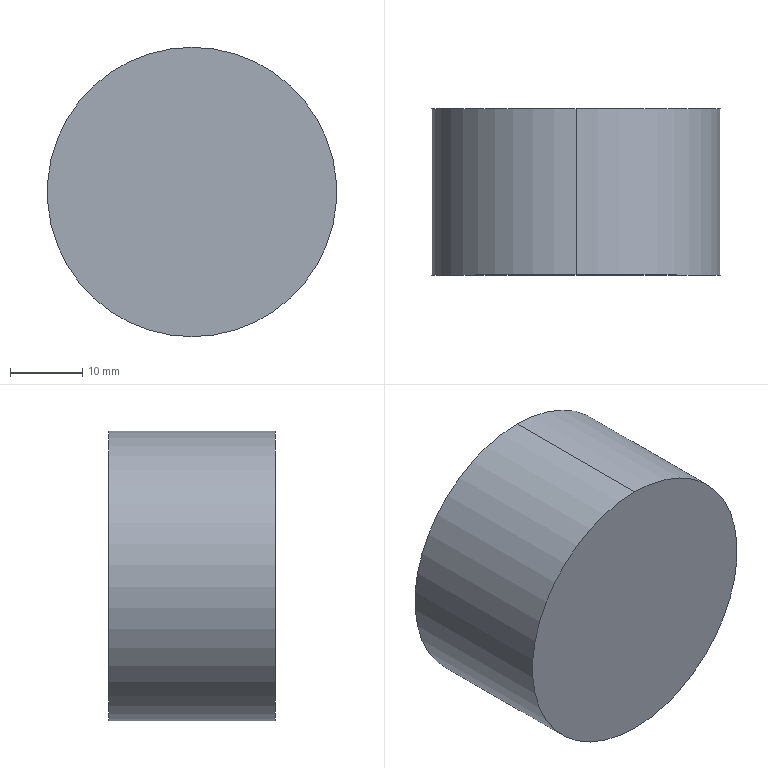Part | 1 solid | 4 faces | box 40 x 23 x 40 mm | volume 28903 mm3 | cylinder 2 | plane 2 | commonest cylinder face diameters 40 x2
STEP:
#1=CARTESIAN_POINT('',(0.,0.,0.));
#2=DIRECTION('',(0.,0.,1.));
#3=DIRECTION('',(1.,0.,0.));
#4=AXIS2_PLACEMENT_3D('',#1,#2,#3);
#5=CARTESIAN_POINT('',(-239.028,-123.5,-320.55));
#6=VERTEX_POINT('',#5);
#7=CARTESIAN_POINT('',(-239.028,-100.5,-320.55));
#8=VERTEX_POINT('',#7);
#9=CARTESIAN_POINT('',(-239.028,-123.5,-320.55));
#10=DIRECTION('',(0.,1.,0.));
#11=VECTOR('',#10,1.);
#12=LINE('',#9,#11);
#13=CARTESIAN_POINT('',(-239.028,-123.5,-300.55));
#14=DIRECTION('',(0.,1.,0.));
#15=DIRECTION('',(1.,0.,0.));
#16=AXIS2_PLACEMENT_3D('',#13,#14,#15);
#17=CYLINDRICAL_SURFACE('',#16,20.);
#18=CARTESIAN_POINT('',(1.571,0.));
#19=DIRECTION('',(0.,1.));
#20=VECTOR('',#19,1.);
#21=LINE('',#18,#20);
#22=(GEOMETRIC_REPRESENTATION_CONTEXT(2)PARAMETRIC_REPRESENTATION_CONTEXT()REPRESENTATION_CONTEXT('',''));
#23=DEFINITIONAL_REPRESENTATION('',(#21),#22);
#24=PCURVE('',#17,#23);
#25=CARTESIAN_POINT('',(-239.028,-123.5,-300.55));
#26=DIRECTION('',(0.,1.,0.));
#27=DIRECTION('',(-1.,0.,0.));
#28=AXIS2_PLACEMENT_3D('',#25,#26,#27);
#29=CYLINDRICAL_SURFACE('',#28,20.);
#30=CARTESIAN_POINT('',(4.712,0.));
#31=DIRECTION('',(0.,1.));
#32=VECTOR('',#31,1.);
#33=LINE('',#30,#32);
#34=(GEOMETRIC_REPRESENTATION_CONTEXT(2)PARAMETRIC_REPRESENTATION_CONTEXT()REPRESENTATION_CONTEXT('',''));
#35=DEFINITIONAL_REPRESENTATION('',(#33),#34);
#36=PCURVE('',#29,#35);
#37=SURFACE_CURVE('',#12,(#24,#36),.PCURVE_S1.);
#38=EDGE_CURVE('',#6,#8,#37,.T.);
#39=ORIENTED_EDGE('',*,*,#38,.F.);
#40=CARTESIAN_POINT('',(-239.028,-123.5,-280.55));
#41=VERTEX_POINT('',#40);
#42=CARTESIAN_POINT('',(-239.028,-123.5,-300.55));
#43=DIRECTION('',(0.,-1.,0.));
#44=DIRECTION('',(0.,0.,1.));
#45=AXIS2_PLACEMENT_3D('',#42,#43,#44);
#46=CIRCLE('',#45,20.);
#47=CARTESIAN_POINT('',(4.712,0.));
#48=DIRECTION('',(-1.,0.));
#49=VECTOR('',#48,1.);
#50=LINE('',#47,#49);
#51=(GEOMETRIC_REPRESENTATION_CONTEXT(2)PARAMETRIC_REPRESENTATION_CONTEXT()REPRESENTATION_CONTEXT('',''));
#52=DEFINITIONAL_REPRESENTATION('',(#50),#51);
#53=PCURVE('',#17,#52);
#54=CARTESIAN_POINT('',(-239.028,-123.5,-300.55));
#55=DIRECTION('',(0.,-1.,0.));
#56=DIRECTION('',(0.,0.,-1.));
#57=AXIS2_PLACEMENT_3D('',#54,#55,#56);
#58=PLANE('',#57);
#59=CARTESIAN_POINT('',(0.,0.));
#60=DIRECTION('',(-1.,0.));
#61=AXIS2_PLACEMENT_2D('',#59,#60);
#62=CIRCLE('',#61,20.);
#63=(GEOMETRIC_REPRESENTATION_CONTEXT(2)PARAMETRIC_REPRESENTATION_CONTEXT()REPRESENTATION_CONTEXT('',''));
#64=DEFINITIONAL_REPRESENTATION('',(#62),#63);
#65=PCURVE('',#58,#64);
#66=SURFACE_CURVE('',#46,(#53,#65),.PCURVE_S1.);
#67=EDGE_CURVE('',#41,#6,#66,.T.);
#68=ORIENTED_EDGE('',*,*,#67,.F.);
#69=CARTESIAN_POINT('',(-239.028,-100.5,-280.55));
#70=VERTEX_POINT('',#69);
#71=CARTESIAN_POINT('',(-239.028,-123.5,-280.55));
#72=DIRECTION('',(0.,1.,0.));
#73=VECTOR('',#72,1.);
#74=LINE('',#71,#73);
#75=CARTESIAN_POINT('',(4.712,0.));
#76=DIRECTION('',(0.,1.));
#77=VECTOR('',#76,1.);
#78=LINE('',#75,#77);
#79=(GEOMETRIC_REPRESENTATION_CONTEXT(2)PARAMETRIC_REPRESENTATION_CONTEXT()REPRESENTATION_CONTEXT('',''));
#80=DEFINITIONAL_REPRESENTATION('',(#78),#79);
#81=PCURVE('',#17,#80);
#82=CARTESIAN_POINT('',(1.571,0.));
#83=DIRECTION('',(0.,1.));
#84=VECTOR('',#83,1.);
#85=LINE('',#82,#84);
#86=(GEOMETRIC_REPRESENTATION_CONTEXT(2)PARAMETRIC_REPRESENTATION_CONTEXT()REPRESENTATION_CONTEXT('',''));
#87=DEFINITIONAL_REPRESENTATION('',(#85),#86);
#88=PCURVE('',#29,#87);
#89=SURFACE_CURVE('',#74,(#81,#88),.PCURVE_S1.);
#90=EDGE_CURVE('',#41,#70,#89,.T.);
#91=ORIENTED_EDGE('',*,*,#90,.T.);
#92=CARTESIAN_POINT('',(-239.028,-100.5,-300.55));
#93=DIRECTION('',(0.,-1.,0.));
#94=DIRECTION('',(0.,0.,1.));
#95=AXIS2_PLACEMENT_3D('',#92,#93,#94);
#96=CIRCLE('',#95,20.);
#97=CARTESIAN_POINT('',(4.712,23.));
#98=DIRECTION('',(-1.,0.));
#99=VECTOR('',#98,1.);
#100=LINE('',#97,#99);
#101=(GEOMETRIC_REPRESENTATION_CONTEXT(2)PARAMETRIC_REPRESENTATION_CONTEXT()REPRESENTATION_CONTEXT('',''));
#102=DEFINITIONAL_REPRESENTATION('',(#100),#101);
#103=PCURVE('',#17,#102);
#104=CARTESIAN_POINT('',(-239.028,-100.5,-300.55));
#105=DIRECTION('',(0.,-1.,0.));
#106=DIRECTION('',(0.,0.,-1.));
#107=AXIS2_PLACEMENT_3D('',#104,#105,#106);
#108=PLANE('',#107);
#109=CARTESIAN_POINT('',(0.,0.));
#110=DIRECTION('',(-1.,0.));
#111=AXIS2_PLACEMENT_2D('',#109,#110);
#112=CIRCLE('',#111,20.);
#113=(GEOMETRIC_REPRESENTATION_CONTEXT(2)PARAMETRIC_REPRESENTATION_CONTEXT()REPRESENTATION_CONTEXT('',''));
#114=DEFINITIONAL_REPRESENTATION('',(#112),#113);
#115=PCURVE('',#108,#114);
#116=SURFACE_CURVE('',#96,(#103,#115),.PCURVE_S1.);
#117=EDGE_CURVE('',#70,#8,#116,.T.);
#118=ORIENTED_EDGE('',*,*,#117,.T.);
#119=EDGE_LOOP('',(#39,#68,#91,#118));
#120=FACE_BOUND('',#119,.T.);
#121=ADVANCED_FACE('',(#120),#17,.T.);
#122=ORIENTED_EDGE('',*,*,#67,.T.);
#123=CARTESIAN_POINT('',(-239.028,-123.5,-300.55));
#124=DIRECTION('',(0.,-1.,0.));
#125=DIRECTION('',(0.,0.,1.));
#126=AXIS2_PLACEMENT_3D('',#123,#124,#125);
#127=CIRCLE('',#126,20.);
#128=CARTESIAN_POINT('',(0.,0.));
#129=DIRECTION('',(-1.,0.));
#130=AXIS2_PLACEMENT_2D('',#128,#129);
#131=CIRCLE('',#130,20.);
#132=(GEOMETRIC_REPRESENTATION_CONTEXT(2)PARAMETRIC_REPRESENTATION_CONTEXT()REPRESENTATION_CONTEXT('',''));
#133=DEFINITIONAL_REPRESENTATION('',(#131),#132);
#134=PCURVE('',#58,#133);
#135=CARTESIAN_POINT('',(7.854,0.));
#136=DIRECTION('',(-1.,0.));
#137=VECTOR('',#136,1.);
#138=LINE('',#135,#137);
#139=(GEOMETRIC_REPRESENTATION_CONTEXT(2)PARAMETRIC_REPRESENTATION_CONTEXT()REPRESENTATION_CONTEXT('',''));
#140=DEFINITIONAL_REPRESENTATION('',(#138),#139);
#141=PCURVE('',#29,#140);
#142=SURFACE_CURVE('',#127,(#134,#141),.PCURVE_S1.);
#143=EDGE_CURVE('',#6,#41,#142,.T.);
#144=ORIENTED_EDGE('',*,*,#143,.T.);
#145=EDGE_LOOP('',(#122,#144));
#146=FACE_BOUND('',#145,.T.);
#147=ADVANCED_FACE('',(#146),#58,.T.);
#148=CARTESIAN_POINT('',(-239.028,-100.5,-300.55));
#149=DIRECTION('',(0.,-1.,0.));
#150=DIRECTION('',(0.,0.,1.));
#151=AXIS2_PLACEMENT_3D('',#148,#149,#150);
#152=CIRCLE('',#151,20.);
#153=CARTESIAN_POINT('',(0.,0.));
#154=DIRECTION('',(-1.,0.));
#155=AXIS2_PLACEMENT_2D('',#153,#154);
#156=CIRCLE('',#155,20.);
#157=(GEOMETRIC_REPRESENTATION_CONTEXT(2)PARAMETRIC_REPRESENTATION_CONTEXT()REPRESENTATION_CONTEXT('',''));
#158=DEFINITIONAL_REPRESENTATION('',(#156),#157);
#159=PCURVE('',#108,#158);
#160=CARTESIAN_POINT('',(7.854,23.));
#161=DIRECTION('',(-1.,0.));
#162=VECTOR('',#161,1.);
#163=LINE('',#160,#162);
#164=(GEOMETRIC_REPRESENTATION_CONTEXT(2)PARAMETRIC_REPRESENTATION_CONTEXT()REPRESENTATION_CONTEXT('',''));
#165=DEFINITIONAL_REPRESENTATION('',(#163),#164);
#166=PCURVE('',#29,#165);
#167=SURFACE_CURVE('',#152,(#159,#166),.PCURVE_S1.);
#168=EDGE_CURVE('',#8,#70,#167,.T.);
#169=ORIENTED_EDGE('',*,*,#168,.F.);
#170=ORIENTED_EDGE('',*,*,#117,.F.);
#171=EDGE_LOOP('',(#169,#170));
#172=FACE_BOUND('',#171,.T.);
#173=ADVANCED_FACE('',(#172),#108,.F.);
#174=ORIENTED_EDGE('',*,*,#38,.T.);
#175=ORIENTED_EDGE('',*,*,#168,.T.);
#176=ORIENTED_EDGE('',*,*,#90,.F.);
#177=ORIENTED_EDGE('',*,*,#143,.F.);
#178=EDGE_LOOP('',(#174,#175,#176,#177));
#179=FACE_BOUND('',#178,.T.);
#180=ADVANCED_FACE('',(#179),#29,.T.);
#181=CLOSED_SHELL('',(#121,#147,#173,#180));
#182=MANIFOLD_SOLID_BREP('',#181);
#183=(LENGTH_UNIT()NAMED_UNIT(*)SI_UNIT(.MILLI.,.METRE.));
#184=UNCERTAINTY_MEASURE_WITH_UNIT(LENGTH_MEASURE(0.0000001),#183,'','');
#185=(NAMED_UNIT(*)PLANE_ANGLE_UNIT()SI_UNIT($,.RADIAN.));
#186=(NAMED_UNIT(*)SI_UNIT($,.STERADIAN.)SOLID_ANGLE_UNIT());
#187=(GEOMETRIC_REPRESENTATION_CONTEXT(3)GLOBAL_UNCERTAINTY_ASSIGNED_CONTEXT((#184))GLOBAL_UNIT_ASSIGNED_CONTEXT((#183,#185,#186))REPRESENTATION_CONTEXT('',''));
#188=ADVANCED_BREP_SHAPE_REPRESENTATION('',(#4,#182),#187);